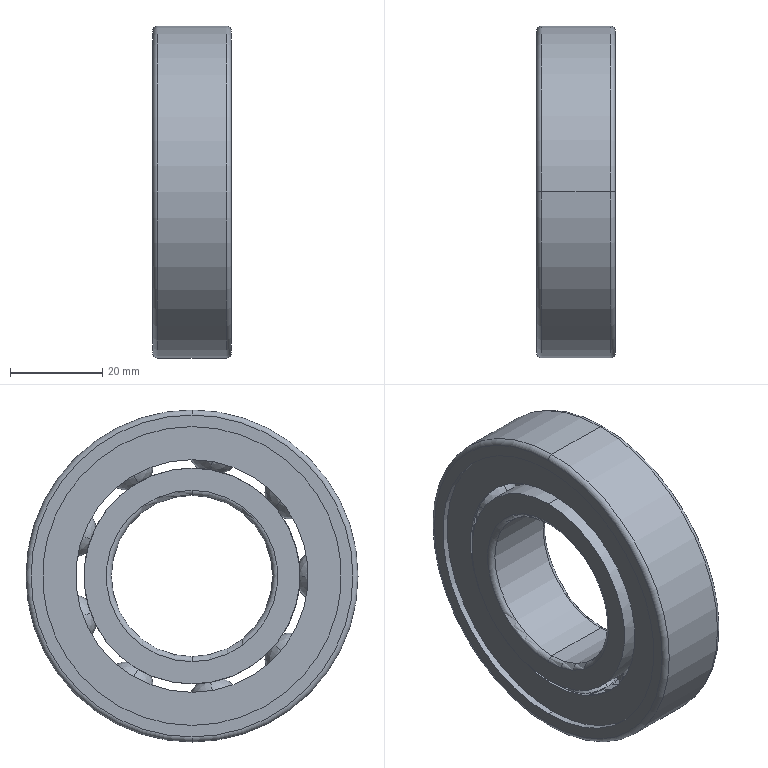Part | NX | features BREP 1 | 1 solid | 199 faces | box 17 x 72 x 72 mm | volume 33160 mm3 | sphere 108 | torus 41 | plane 26 | cylinder 24 | commonest cylinder face diameters 64.8 x8 46.8 x4 50.467 x4 35 x2 52.744 x2 58.856 x2